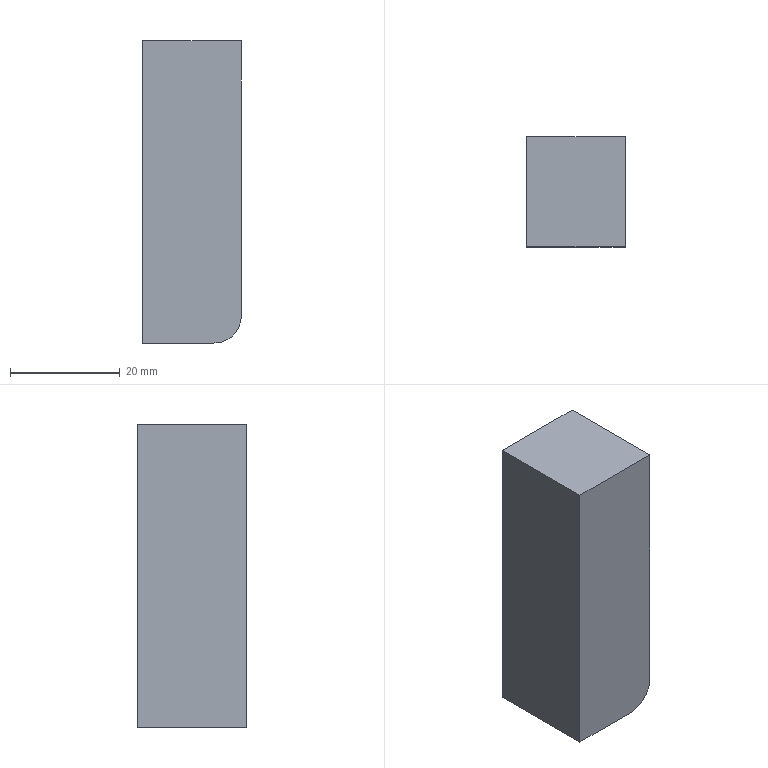Part | STEP file | 1 solid | 7 faces | box 18 x 20 x 55 mm | volume 19693 mm3 | plane 6 | cylinder 1 | commonest cylinder face diameters 10 x1
STEP:
#1=CARTESIAN_POINT('',(0.,0.,0.));
#2=DIRECTION('',(0.,0.,1.));
#3=DIRECTION('',(1.,0.,0.));
#4=AXIS2_PLACEMENT_3D('',#1,#2,#3);
#5=CARTESIAN_POINT('',(-2.862,50.,-37.47));
#6=VERTEX_POINT('',#5);
#7=CARTESIAN_POINT('',(-2.862,70.,-37.47));
#8=VERTEX_POINT('',#7);
#9=CARTESIAN_POINT('',(-2.862,130.5,-37.47));
#10=DIRECTION('',(0.,1.,0.));
#11=VECTOR('',#10,1.);
#12=LINE('',#9,#11);
#13=CARTESIAN_POINT('',(15.138,130.5,-37.47));
#14=DIRECTION('',(0.,0.,1.));
#15=DIRECTION('',(1.,0.,0.));
#16=AXIS2_PLACEMENT_3D('',#13,#14,#15);
#17=PLANE('',#16);
#18=CARTESIAN_POINT('',(-18.,0.));
#19=DIRECTION('',(0.,1.));
#20=VECTOR('',#19,1.);
#21=LINE('',#18,#20);
#22=(GEOMETRIC_REPRESENTATION_CONTEXT(2)PARAMETRIC_REPRESENTATION_CONTEXT()REPRESENTATION_CONTEXT('',''));
#23=DEFINITIONAL_REPRESENTATION('',(#21),#22);
#24=PCURVE('',#17,#23);
#25=CARTESIAN_POINT('',(-2.862,0.,-92.47));
#26=DIRECTION('',(1.,0.,0.));
#27=DIRECTION('',(0.,0.,-1.));
#28=AXIS2_PLACEMENT_3D('',#25,#26,#27);
#29=PLANE('',#28);
#30=CARTESIAN_POINT('',(-55.,130.5));
#31=DIRECTION('',(0.,1.));
#32=VECTOR('',#31,1.);
#33=LINE('',#30,#32);
#34=(GEOMETRIC_REPRESENTATION_CONTEXT(2)PARAMETRIC_REPRESENTATION_CONTEXT()REPRESENTATION_CONTEXT('',''));
#35=DEFINITIONAL_REPRESENTATION('',(#33),#34);
#36=PCURVE('',#29,#35);
#37=SURFACE_CURVE('',#12,(#24,#36),.PCURVE_S1.);
#38=EDGE_CURVE('',#6,#8,#37,.T.);
#39=ORIENTED_EDGE('',*,*,#38,.F.);
#40=CARTESIAN_POINT('',(15.138,50.,-37.47));
#41=VERTEX_POINT('',#40);
#42=CARTESIAN_POINT('',(15.138,50.,-37.47));
#43=DIRECTION('',(-1.,0.,0.));
#44=VECTOR('',#43,1.);
#45=LINE('',#42,#44);
#46=CARTESIAN_POINT('',(0.,-80.5));
#47=DIRECTION('',(-1.,0.));
#48=VECTOR('',#47,1.);
#49=LINE('',#46,#48);
#50=(GEOMETRIC_REPRESENTATION_CONTEXT(2)PARAMETRIC_REPRESENTATION_CONTEXT()REPRESENTATION_CONTEXT('',''));
#51=DEFINITIONAL_REPRESENTATION('',(#49),#50);
#52=PCURVE('',#17,#51);
#53=CARTESIAN_POINT('',(15.138,50.,-92.47));
#54=DIRECTION('',(0.,1.,0.));
#55=DIRECTION('',(0.,0.,1.));
#56=AXIS2_PLACEMENT_3D('',#53,#54,#55);
#57=PLANE('',#56);
#58=CARTESIAN_POINT('',(55.,0.));
#59=DIRECTION('',(0.,-1.));
#60=VECTOR('',#59,1.);
#61=LINE('',#58,#60);
#62=(GEOMETRIC_REPRESENTATION_CONTEXT(2)PARAMETRIC_REPRESENTATION_CONTEXT()REPRESENTATION_CONTEXT('',''));
#63=DEFINITIONAL_REPRESENTATION('',(#61),#62);
#64=PCURVE('',#57,#63);
#65=SURFACE_CURVE('',#45,(#52,#64),.PCURVE_S1.);
#66=EDGE_CURVE('',#41,#6,#65,.T.);
#67=ORIENTED_EDGE('',*,*,#66,.F.);
#68=CARTESIAN_POINT('',(15.138,70.,-37.47));
#69=VERTEX_POINT('',#68);
#70=CARTESIAN_POINT('',(15.138,130.5,-37.47));
#71=DIRECTION('',(0.,1.,0.));
#72=VECTOR('',#71,1.);
#73=LINE('',#70,#72);
#74=CARTESIAN_POINT('',(0.,0.));
#75=DIRECTION('',(0.,1.));
#76=VECTOR('',#75,1.);
#77=LINE('',#74,#76);
#78=(GEOMETRIC_REPRESENTATION_CONTEXT(2)PARAMETRIC_REPRESENTATION_CONTEXT()REPRESENTATION_CONTEXT('',''));
#79=DEFINITIONAL_REPRESENTATION('',(#77),#78);
#80=PCURVE('',#17,#79);
#81=CARTESIAN_POINT('',(15.138,0.,-92.47));
#82=DIRECTION('',(1.,0.,0.));
#83=DIRECTION('',(0.,0.,-1.));
#84=AXIS2_PLACEMENT_3D('',#81,#82,#83);
#85=PLANE('',#84);
#86=CARTESIAN_POINT('',(-55.,130.5));
#87=DIRECTION('',(0.,1.));
#88=VECTOR('',#87,1.);
#89=LINE('',#86,#88);
#90=(GEOMETRIC_REPRESENTATION_CONTEXT(2)PARAMETRIC_REPRESENTATION_CONTEXT()REPRESENTATION_CONTEXT('',''));
#91=DEFINITIONAL_REPRESENTATION('',(#89),#90);
#92=PCURVE('',#85,#91);
#93=SURFACE_CURVE('',#73,(#80,#92),.PCURVE_S1.);
#94=EDGE_CURVE('',#41,#69,#93,.T.);
#95=ORIENTED_EDGE('',*,*,#94,.T.);
#96=CARTESIAN_POINT('',(15.138,70.,-37.47));
#97=DIRECTION('',(-1.,0.,0.));
#98=VECTOR('',#97,1.);
#99=LINE('',#96,#98);
#100=CARTESIAN_POINT('',(0.,-60.5));
#101=DIRECTION('',(-1.,0.));
#102=VECTOR('',#101,1.);
#103=LINE('',#100,#102);
#104=(GEOMETRIC_REPRESENTATION_CONTEXT(2)PARAMETRIC_REPRESENTATION_CONTEXT()REPRESENTATION_CONTEXT('',''));
#105=DEFINITIONAL_REPRESENTATION('',(#103),#104);
#106=PCURVE('',#17,#105);
#107=CARTESIAN_POINT('',(15.138,70.,-92.47));
#108=DIRECTION('',(0.,-1.,0.));
#109=DIRECTION('',(0.,0.,-1.));
#110=AXIS2_PLACEMENT_3D('',#107,#108,#109);
#111=PLANE('',#110);
#112=CARTESIAN_POINT('',(-55.,0.));
#113=DIRECTION('',(0.,-1.));
#114=VECTOR('',#113,1.);
#115=LINE('',#112,#114);
#116=(GEOMETRIC_REPRESENTATION_CONTEXT(2)PARAMETRIC_REPRESENTATION_CONTEXT()REPRESENTATION_CONTEXT('',''));
#117=DEFINITIONAL_REPRESENTATION('',(#115),#116);
#118=PCURVE('',#111,#117);
#119=SURFACE_CURVE('',#99,(#106,#118),.PCURVE_S1.);
#120=EDGE_CURVE('',#69,#8,#119,.T.);
#121=ORIENTED_EDGE('',*,*,#120,.T.);
#122=EDGE_LOOP('',(#39,#67,#95,#121));
#123=FACE_BOUND('',#122,.T.);
#124=ADVANCED_FACE('',(#123),#17,.T.);
#125=CARTESIAN_POINT('',(15.138,70.,-87.47));
#126=VERTEX_POINT('',#125);
#127=CARTESIAN_POINT('',(15.138,70.,-92.47));
#128=DIRECTION('',(0.,0.,1.));
#129=VECTOR('',#128,1.);
#130=LINE('',#127,#129);
#131=CARTESIAN_POINT('',(0.,0.));
#132=DIRECTION('',(-1.,0.));
#133=VECTOR('',#132,1.);
#134=LINE('',#131,#133);
#135=(GEOMETRIC_REPRESENTATION_CONTEXT(2)PARAMETRIC_REPRESENTATION_CONTEXT()REPRESENTATION_CONTEXT('',''));
#136=DEFINITIONAL_REPRESENTATION('',(#134),#135);
#137=PCURVE('',#111,#136);
#138=CARTESIAN_POINT('',(0.,70.));
#139=DIRECTION('',(-1.,0.));
#140=VECTOR('',#139,1.);
#141=LINE('',#138,#140);
#142=(GEOMETRIC_REPRESENTATION_CONTEXT(2)PARAMETRIC_REPRESENTATION_CONTEXT()REPRESENTATION_CONTEXT('',''));
#143=DEFINITIONAL_REPRESENTATION('',(#141),#142);
#144=PCURVE('',#85,#143);
#145=SURFACE_CURVE('',#130,(#137,#144),.PCURVE_S1.);
#146=EDGE_CURVE('',#126,#69,#145,.T.);
#147=ORIENTED_EDGE('',*,*,#146,.F.);
#148=CARTESIAN_POINT('',(10.138,70.,-92.47));
#149=VERTEX_POINT('',#148);
#150=CARTESIAN_POINT('',(10.138,70.,-87.47));
#151=DIRECTION('',(0.,1.,0.));
#152=DIRECTION('',(0.,0.,-1.));
#153=AXIS2_PLACEMENT_3D('',#150,#151,#152);
#154=CIRCLE('',#153,5.);
#155=CARTESIAN_POINT('',(0.,-5.));
#156=CARTESIAN_POINT('',(0.,-13.66));
#157=CARTESIAN_POINT('',(-7.5,-9.33));
#158=CARTESIAN_POINT('',(-15.,-5.));
#159=CARTESIAN_POINT('',(-7.5,-0.6699));
#160=CARTESIAN_POINT('',(0.,3.66));
#161=CARTESIAN_POINT('',(0.,-5.));
#162=(BOUNDED_CURVE()B_SPLINE_CURVE(2,(#155,#156,#157,#158,#159,#160,#161),.UNSPECIFIED.,.T.,.F.)B_SPLINE_CURVE_WITH_KNOTS((1,2,2,2,2,1),(-2.094,0.,2.094,4.189,6.283,8.378),.UNSPECIFIED.)CURVE()GEOMETRIC_REPRESENTATION_ITEM()RATIONAL_B_SPLINE_CURVE((1.,0.5,1.,0.5,1.,0.5,1.))REPRESENTATION_ITEM(''));
#163=(GEOMETRIC_REPRESENTATION_CONTEXT(2)PARAMETRIC_REPRESENTATION_CONTEXT()REPRESENTATION_CONTEXT('',''));
#164=DEFINITIONAL_REPRESENTATION('',(#162),#163);
#165=PCURVE('',#111,#164);
#166=CARTESIAN_POINT('',(10.138,0.,-87.47));
#167=DIRECTION('',(0.,-1.,0.));
#168=DIRECTION('',(0.,0.,-1.));
#169=AXIS2_PLACEMENT_3D('',#166,#167,#168);
#170=CYLINDRICAL_SURFACE('',#169,5.);
#171=CARTESIAN_POINT('',(6.283,-70.));
#172=DIRECTION('',(-1.,0.));
#173=VECTOR('',#172,1.);
#174=LINE('',#171,#173);
#175=(GEOMETRIC_REPRESENTATION_CONTEXT(2)PARAMETRIC_REPRESENTATION_CONTEXT()REPRESENTATION_CONTEXT('',''));
#176=DEFINITIONAL_REPRESENTATION('',(#174),#175);
#177=PCURVE('',#170,#176);
#178=SURFACE_CURVE('',#154,(#165,#177),.PCURVE_S1.);
#179=EDGE_CURVE('',#126,#149,#178,.T.);
#180=ORIENTED_EDGE('',*,*,#179,.T.);
#181=CARTESIAN_POINT('',(-2.862,70.,-92.47));
#182=VERTEX_POINT('',#181);
#183=CARTESIAN_POINT('',(15.138,70.,-92.47));
#184=DIRECTION('',(-1.,0.,0.));
#185=VECTOR('',#184,1.);
#186=LINE('',#183,#185);
#187=CARTESIAN_POINT('',(0.,0.));
#188=DIRECTION('',(0.,-1.));
#189=VECTOR('',#188,1.);
#190=LINE('',#187,#189);
#191=(GEOMETRIC_REPRESENTATION_CONTEXT(2)PARAMETRIC_REPRESENTATION_CONTEXT()REPRESENTATION_CONTEXT('',''));
#192=DEFINITIONAL_REPRESENTATION('',(#190),#191);
#193=PCURVE('',#111,#192);
#194=CARTESIAN_POINT('',(15.138,0.,-92.47));
#195=DIRECTION('',(0.,0.,1.));
#196=DIRECTION('',(1.,0.,0.));
#197=AXIS2_PLACEMENT_3D('',#194,#195,#196);
#198=PLANE('',#197);
#199=CARTESIAN_POINT('',(0.,70.));
#200=DIRECTION('',(-1.,0.));
#201=VECTOR('',#200,1.);
#202=LINE('',#199,#201);
#203=(GEOMETRIC_REPRESENTATION_CONTEXT(2)PARAMETRIC_REPRESENTATION_CONTEXT()REPRESENTATION_CONTEXT('',''));
#204=DEFINITIONAL_REPRESENTATION('',(#202),#203);
#205=PCURVE('',#198,#204);
#206=SURFACE_CURVE('',#186,(#193,#205),.PCURVE_S1.);
#207=EDGE_CURVE('',#149,#182,#206,.T.);
#208=ORIENTED_EDGE('',*,*,#207,.T.);
#209=CARTESIAN_POINT('',(-2.862,70.,-92.47));
#210=DIRECTION('',(0.,0.,1.));
#211=VECTOR('',#210,1.);
#212=LINE('',#209,#211);
#213=CARTESIAN_POINT('',(0.,-18.));
#214=DIRECTION('',(-1.,0.));
#215=VECTOR('',#214,1.);
#216=LINE('',#213,#215);
#217=(GEOMETRIC_REPRESENTATION_CONTEXT(2)PARAMETRIC_REPRESENTATION_CONTEXT()REPRESENTATION_CONTEXT('',''));
#218=DEFINITIONAL_REPRESENTATION('',(#216),#217);
#219=PCURVE('',#111,#218);
#220=CARTESIAN_POINT('',(0.,70.));
#221=DIRECTION('',(-1.,0.));
#222=VECTOR('',#221,1.);
#223=LINE('',#220,#222);
#224=(GEOMETRIC_REPRESENTATION_CONTEXT(2)PARAMETRIC_REPRESENTATION_CONTEXT()REPRESENTATION_CONTEXT('',''));
#225=DEFINITIONAL_REPRESENTATION('',(#223),#224);
#226=PCURVE('',#29,#225);
#227=SURFACE_CURVE('',#212,(#219,#226),.PCURVE_S1.);
#228=EDGE_CURVE('',#182,#8,#227,.T.);
#229=ORIENTED_EDGE('',*,*,#228,.T.);
#230=ORIENTED_EDGE('',*,*,#120,.F.);
#231=EDGE_LOOP('',(#147,#180,#208,#229,#230));
#232=FACE_BOUND('',#231,.T.);
#233=ADVANCED_FACE('',(#232),#111,.F.);
#234=ORIENTED_EDGE('',*,*,#207,.F.);
#235=CARTESIAN_POINT('',(10.138,50.,-92.47));
#236=VERTEX_POINT('',#235);
#237=CARTESIAN_POINT('',(10.138,50.,-92.47));
#238=DIRECTION('',(0.,-1.,0.));
#239=VECTOR('',#238,1.);
#240=LINE('',#237,#239);
#241=CARTESIAN_POINT('',(-5.,50.));
#242=DIRECTION('',(0.,-1.));
#243=VECTOR('',#242,1.);
#244=LINE('',#241,#243);
#245=(GEOMETRIC_REPRESENTATION_CONTEXT(2)PARAMETRIC_REPRESENTATION_CONTEXT()REPRESENTATION_CONTEXT('',''));
#246=DEFINITIONAL_REPRESENTATION('',(#244),#245);
#247=PCURVE('',#198,#246);
#248=CARTESIAN_POINT('',(0.,-50.));
#249=DIRECTION('',(0.,1.));
#250=VECTOR('',#249,1.);
#251=LINE('',#248,#250);
#252=(GEOMETRIC_REPRESENTATION_CONTEXT(2)PARAMETRIC_REPRESENTATION_CONTEXT()REPRESENTATION_CONTEXT('',''));
#253=DEFINITIONAL_REPRESENTATION('',(#251),#252);
#254=PCURVE('',#170,#253);
#255=SURFACE_CURVE('',#240,(#247,#254),.PCURVE_S1.);
#256=EDGE_CURVE('',#149,#236,#255,.T.);
#257=ORIENTED_EDGE('',*,*,#256,.T.);
#258=CARTESIAN_POINT('',(-2.862,50.,-92.47));
#259=VERTEX_POINT('',#258);
#260=CARTESIAN_POINT('',(10.138,50.,-92.47));
#261=CARTESIAN_POINT('',(5.804,50.,-92.47));
#262=CARTESIAN_POINT('',(1.471,50.,-92.47));
#263=CARTESIAN_POINT('',(-2.862,50.,-92.47));
#264=B_SPLINE_CURVE_WITH_KNOTS('',3,(#260,#261,#262,#263),.UNSPECIFIED.,.F.,.F.,(4,4),(0.2778,1.),.PIECEWISE_BEZIER_KNOTS.);
#265=CARTESIAN_POINT('',(-5.,50.));
#266=CARTESIAN_POINT('',(-9.333,50.));
#267=CARTESIAN_POINT('',(-13.667,50.));
#268=CARTESIAN_POINT('',(-18.,50.));
#269=B_SPLINE_CURVE_WITH_KNOTS('',3,(#265,#266,#267,#268),.UNSPECIFIED.,.F.,.F.,(4,4),(0.2778,1.),.PIECEWISE_BEZIER_KNOTS.);
#270=(GEOMETRIC_REPRESENTATION_CONTEXT(2)PARAMETRIC_REPRESENTATION_CONTEXT()REPRESENTATION_CONTEXT('',''));
#271=DEFINITIONAL_REPRESENTATION('',(#269),#270);
#272=PCURVE('',#198,#271);
#273=CARTESIAN_POINT('',(0.,-5.));
#274=CARTESIAN_POINT('',(0.,-9.333));
#275=CARTESIAN_POINT('',(0.,-13.667));
#276=CARTESIAN_POINT('',(0.,-18.));
#277=B_SPLINE_CURVE_WITH_KNOTS('',3,(#273,#274,#275,#276),.UNSPECIFIED.,.F.,.F.,(4,4),(0.2778,1.),.PIECEWISE_BEZIER_KNOTS.);
#278=(GEOMETRIC_REPRESENTATION_CONTEXT(2)PARAMETRIC_REPRESENTATION_CONTEXT()REPRESENTATION_CONTEXT('',''));
#279=DEFINITIONAL_REPRESENTATION('',(#277),#278);
#280=PCURVE('',#57,#279);
#281=SURFACE_CURVE('',#264,(#272,#280),.PCURVE_S1.);
#282=EDGE_CURVE('',#236,#259,#281,.T.);
#283=ORIENTED_EDGE('',*,*,#282,.T.);
#284=CARTESIAN_POINT('',(-2.862,0.,-92.47));
#285=DIRECTION('',(0.,1.,0.));
#286=VECTOR('',#285,1.);
#287=LINE('',#284,#286);
#288=CARTESIAN_POINT('',(-18.,0.));
#289=DIRECTION('',(0.,1.));
#290=VECTOR('',#289,1.);
#291=LINE('',#288,#290);
#292=(GEOMETRIC_REPRESENTATION_CONTEXT(2)PARAMETRIC_REPRESENTATION_CONTEXT()REPRESENTATION_CONTEXT('',''));
#293=DEFINITIONAL_REPRESENTATION('',(#291),#292);
#294=PCURVE('',#198,#293);
#295=CARTESIAN_POINT('',(0.,0.));
#296=DIRECTION('',(0.,1.));
#297=VECTOR('',#296,1.);
#298=LINE('',#295,#297);
#299=(GEOMETRIC_REPRESENTATION_CONTEXT(2)PARAMETRIC_REPRESENTATION_CONTEXT()REPRESENTATION_CONTEXT('',''));
#300=DEFINITIONAL_REPRESENTATION('',(#298),#299);
#301=PCURVE('',#29,#300);
#302=SURFACE_CURVE('',#287,(#294,#301),.PCURVE_S1.);
#303=EDGE_CURVE('',#259,#182,#302,.T.);
#304=ORIENTED_EDGE('',*,*,#303,.T.);
#305=EDGE_LOOP('',(#234,#257,#283,#304));
#306=FACE_BOUND('',#305,.T.);
#307=ADVANCED_FACE('',(#306),#198,.F.);
#308=ORIENTED_EDGE('',*,*,#282,.F.);
#309=CARTESIAN_POINT('',(15.138,50.,-87.47));
#310=VERTEX_POINT('',#309);
#311=CARTESIAN_POINT('',(10.138,50.,-87.47));
#312=DIRECTION('',(0.,-1.,0.));
#313=DIRECTION('',(0.,0.,1.));
#314=AXIS2_PLACEMENT_3D('',#311,#312,#313);
#315=CIRCLE('',#314,5.);
#316=CARTESIAN_POINT('',(10.,-5.));
#317=CARTESIAN_POINT('',(10.,-13.66));
#318=CARTESIAN_POINT('',(2.5,-9.33));
#319=CARTESIAN_POINT('',(-5.,-5.));
#320=CARTESIAN_POINT('',(2.5,-0.6699));
#321=CARTESIAN_POINT('',(10.,3.66));
#322=CARTESIAN_POINT('',(10.,-5.));
#323=(BOUNDED_CURVE()B_SPLINE_CURVE(2,(#316,#317,#318,#319,#320,#321,#322),.UNSPECIFIED.,.T.,.F.)B_SPLINE_CURVE_WITH_KNOTS((1,2,2,2,2,1),(-2.094,0.,2.094,4.189,6.283,8.378),.UNSPECIFIED.)CURVE()GEOMETRIC_REPRESENTATION_ITEM()RATIONAL_B_SPLINE_CURVE((1.,0.5,1.,0.5,1.,0.5,1.))REPRESENTATION_ITEM(''));
#324=(GEOMETRIC_REPRESENTATION_CONTEXT(2)PARAMETRIC_REPRESENTATION_CONTEXT()REPRESENTATION_CONTEXT('',''));
#325=DEFINITIONAL_REPRESENTATION('',(#323),#324);
#326=PCURVE('',#57,#325);
#327=CARTESIAN_POINT('',(-3.142,-50.));
#328=DIRECTION('',(1.,0.));
#329=VECTOR('',#328,1.);
#330=LINE('',#327,#329);
#331=(GEOMETRIC_REPRESENTATION_CONTEXT(2)PARAMETRIC_REPRESENTATION_CONTEXT()REPRESENTATION_CONTEXT('',''));
#332=DEFINITIONAL_REPRESENTATION('',(#330),#331);
#333=PCURVE('',#170,#332);
#334=SURFACE_CURVE('',#315,(#326,#333),.PCURVE_S1.);
#335=EDGE_CURVE('',#236,#310,#334,.T.);
#336=ORIENTED_EDGE('',*,*,#335,.T.);
#337=CARTESIAN_POINT('',(15.138,50.,-92.47));
#338=DIRECTION('',(0.,0.,-1.));
#339=VECTOR('',#338,1.);
#340=LINE('',#337,#339);
#341=CARTESIAN_POINT('',(0.,0.));
#342=DIRECTION('',(-1.,0.));
#343=VECTOR('',#342,1.);
#344=LINE('',#341,#343);
#345=(GEOMETRIC_REPRESENTATION_CONTEXT(2)PARAMETRIC_REPRESENTATION_CONTEXT()REPRESENTATION_CONTEXT('',''));
#346=DEFINITIONAL_REPRESENTATION('',(#344),#345);
#347=PCURVE('',#57,#346);
#348=CARTESIAN_POINT('',(0.,50.));
#349=DIRECTION('',(1.,0.));
#350=VECTOR('',#349,1.);
#351=LINE('',#348,#350);
#352=(GEOMETRIC_REPRESENTATION_CONTEXT(2)PARAMETRIC_REPRESENTATION_CONTEXT()REPRESENTATION_CONTEXT('',''));
#353=DEFINITIONAL_REPRESENTATION('',(#351),#352);
#354=PCURVE('',#85,#353);
#355=SURFACE_CURVE('',#340,(#347,#354),.PCURVE_S1.);
#356=EDGE_CURVE('',#41,#310,#355,.T.);
#357=ORIENTED_EDGE('',*,*,#356,.F.);
#358=ORIENTED_EDGE('',*,*,#66,.T.);
#359=CARTESIAN_POINT('',(-2.862,50.,-92.47));
#360=DIRECTION('',(0.,0.,-1.));
#361=VECTOR('',#360,1.);
#362=LINE('',#359,#361);
#363=CARTESIAN_POINT('',(0.,-18.));
#364=DIRECTION('',(-1.,0.));
#365=VECTOR('',#364,1.);
#366=LINE('',#363,#365);
#367=(GEOMETRIC_REPRESENTATION_CONTEXT(2)PARAMETRIC_REPRESENTATION_CONTEXT()REPRESENTATION_CONTEXT('',''));
#368=DEFINITIONAL_REPRESENTATION('',(#366),#367);
#369=PCURVE('',#57,#368);
#370=CARTESIAN_POINT('',(0.,50.));
#371=DIRECTION('',(1.,0.));
#372=VECTOR('',#371,1.);
#373=LINE('',#370,#372);
#374=(GEOMETRIC_REPRESENTATION_CONTEXT(2)PARAMETRIC_REPRESENTATION_CONTEXT()REPRESENTATION_CONTEXT('',''));
#375=DEFINITIONAL_REPRESENTATION('',(#373),#374);
#376=PCURVE('',#29,#375);
#377=SURFACE_CURVE('',#362,(#369,#376),.PCURVE_S1.);
#378=EDGE_CURVE('',#6,#259,#377,.T.);
#379=ORIENTED_EDGE('',*,*,#378,.T.);
#380=EDGE_LOOP('',(#308,#336,#357,#358,#379));
#381=FACE_BOUND('',#380,.T.);
#382=ADVANCED_FACE('',(#381),#57,.F.);
#383=ORIENTED_EDGE('',*,*,#356,.T.);
#384=CARTESIAN_POINT('',(15.138,70.,-87.47));
#385=DIRECTION('',(0.,1.,0.));
#386=VECTOR('',#385,1.);
#387=LINE('',#384,#386);
#388=CARTESIAN_POINT('',(-5.,70.));
#389=DIRECTION('',(0.,1.));
#390=VECTOR('',#389,1.);
#391=LINE('',#388,#390);
#392=(GEOMETRIC_REPRESENTATION_CONTEXT(2)PARAMETRIC_REPRESENTATION_CONTEXT()REPRESENTATION_CONTEXT('',''));
#393=DEFINITIONAL_REPRESENTATION('',(#391),#392);
#394=PCURVE('',#85,#393);
#395=CARTESIAN_POINT('',(1.571,-70.));
#396=DIRECTION('',(0.,-1.));
#397=VECTOR('',#396,1.);
#398=LINE('',#395,#397);
#399=(GEOMETRIC_REPRESENTATION_CONTEXT(2)PARAMETRIC_REPRESENTATION_CONTEXT()REPRESENTATION_CONTEXT('',''));
#400=DEFINITIONAL_REPRESENTATION('',(#398),#399);
#401=PCURVE('',#170,#400);
#402=SURFACE_CURVE('',#387,(#394,#401),.PCURVE_S1.);
#403=EDGE_CURVE('',#310,#126,#402,.T.);
#404=ORIENTED_EDGE('',*,*,#403,.T.);
#405=ORIENTED_EDGE('',*,*,#146,.T.);
#406=ORIENTED_EDGE('',*,*,#94,.F.);
#407=EDGE_LOOP('',(#383,#404,#405,#406));
#408=FACE_BOUND('',#407,.T.);
#409=ADVANCED_FACE('',(#408),#85,.T.);
#410=ORIENTED_EDGE('',*,*,#38,.T.);
#411=ORIENTED_EDGE('',*,*,#228,.F.);
#412=ORIENTED_EDGE('',*,*,#303,.F.);
#413=ORIENTED_EDGE('',*,*,#378,.F.);
#414=EDGE_LOOP('',(#410,#411,#412,#413));
#415=FACE_BOUND('',#414,.T.);
#416=ADVANCED_FACE('',(#415),#29,.F.);
#417=ORIENTED_EDGE('',*,*,#335,.F.);
#418=ORIENTED_EDGE('',*,*,#256,.F.);
#419=ORIENTED_EDGE('',*,*,#179,.F.);
#420=ORIENTED_EDGE('',*,*,#403,.F.);
#421=EDGE_LOOP('',(#417,#418,#419,#420));
#422=FACE_BOUND('',#421,.T.);
#423=ADVANCED_FACE('',(#422),#170,.T.);
#424=CLOSED_SHELL('',(#124,#233,#307,#382,#409,#416,#423));
#425=MANIFOLD_SOLID_BREP('',#424);
#426=(LENGTH_UNIT()NAMED_UNIT(*)SI_UNIT(.MILLI.,.METRE.));
#427=UNCERTAINTY_MEASURE_WITH_UNIT(LENGTH_MEASURE(0.0000001),#426,'','');
#428=(NAMED_UNIT(*)PLANE_ANGLE_UNIT()SI_UNIT($,.RADIAN.));
#429=(NAMED_UNIT(*)SI_UNIT($,.STERADIAN.)SOLID_ANGLE_UNIT());
#430=(GEOMETRIC_REPRESENTATION_CONTEXT(3)GLOBAL_UNCERTAINTY_ASSIGNED_CONTEXT((#427))GLOBAL_UNIT_ASSIGNED_CONTEXT((#426,#428,#429))REPRESENTATION_CONTEXT('',''));
#431=ADVANCED_BREP_SHAPE_REPRESENTATION('',(#4,#425),#430);